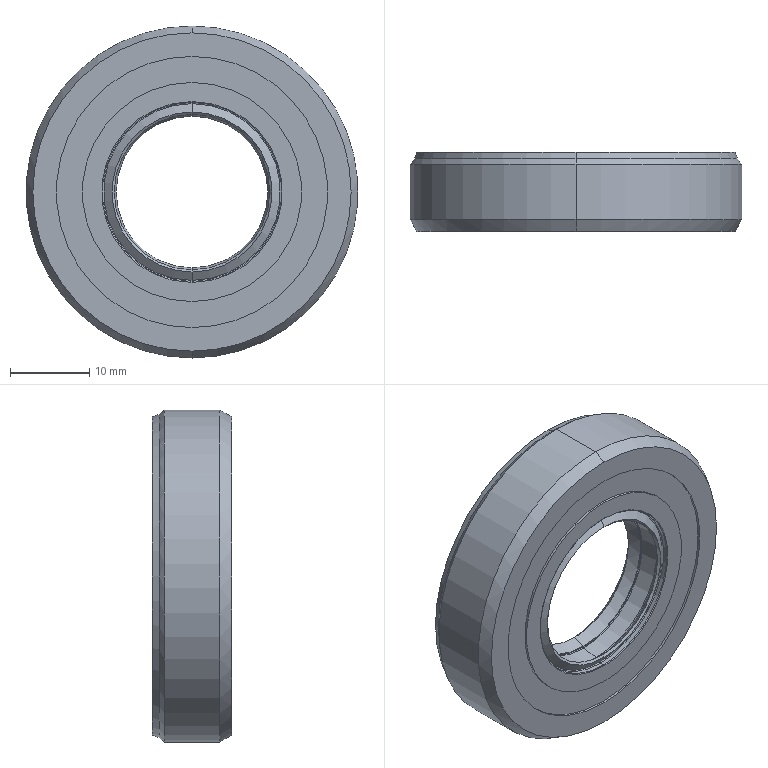Part | SolidWorks | features BaseBody 3 | 3 solids | 85 faces | box 42 x 10 x 42 mm | volume 3936 mm3 | torus 24 | cylinder 24 | cone 22 | plane 15 | commonest cylinder face diameters 39 x6 23.5 x4 40.8 x4 22.668 x2 26.505 x2 27.7 x2